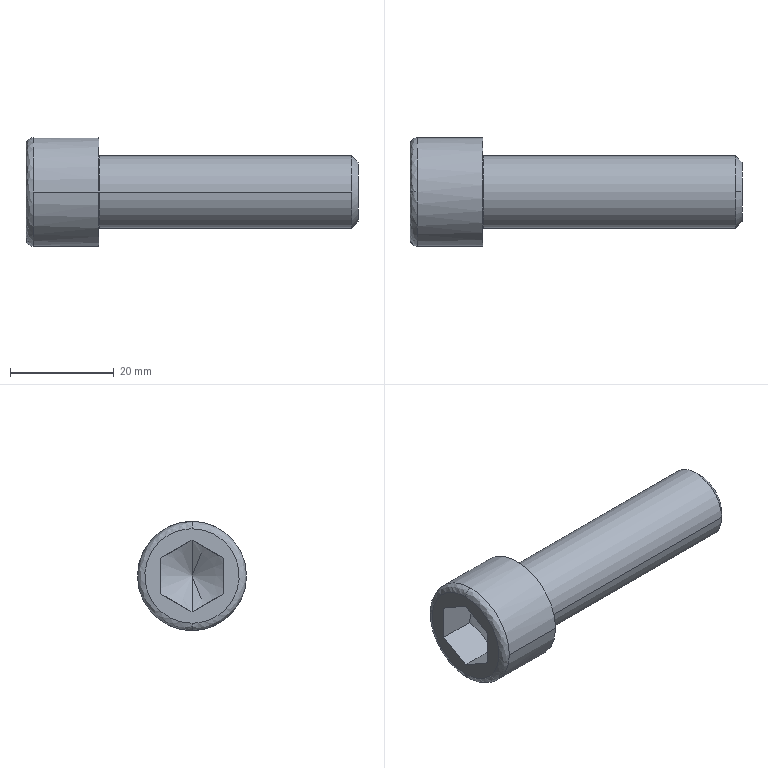Part | STEP file | DIN 912 - replaced by DIN EN ISO 4762 M14 x 50 | 1 solid | 21 faces | box 64 x 21 x 21 mm | volume 11420 mm3 | plane 9 | spline 4 | cylinder 4 | cone 4 | commonest cylinder face diameters 14 x2 21 x2